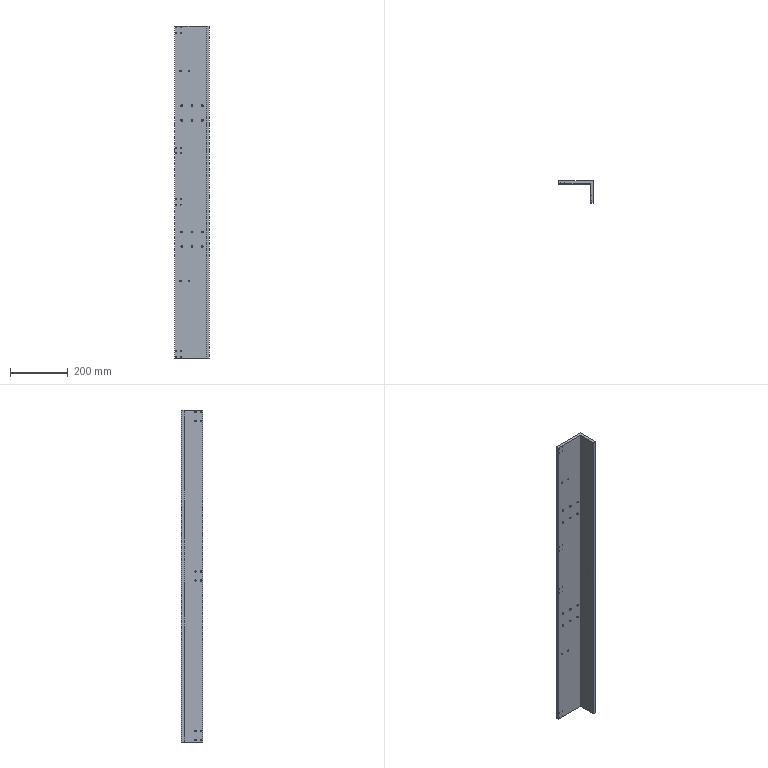Part | SolidWorks | features HoleWzd 4, Extrusion 1 | 1 solid | 96 faces | box 120 x 75 x 1150 mm | volume 2118632 mm3 | cylinder 88 | plane 8 | commonest cylinder face diameters 3.3 x32 5 x32 6.8 x24